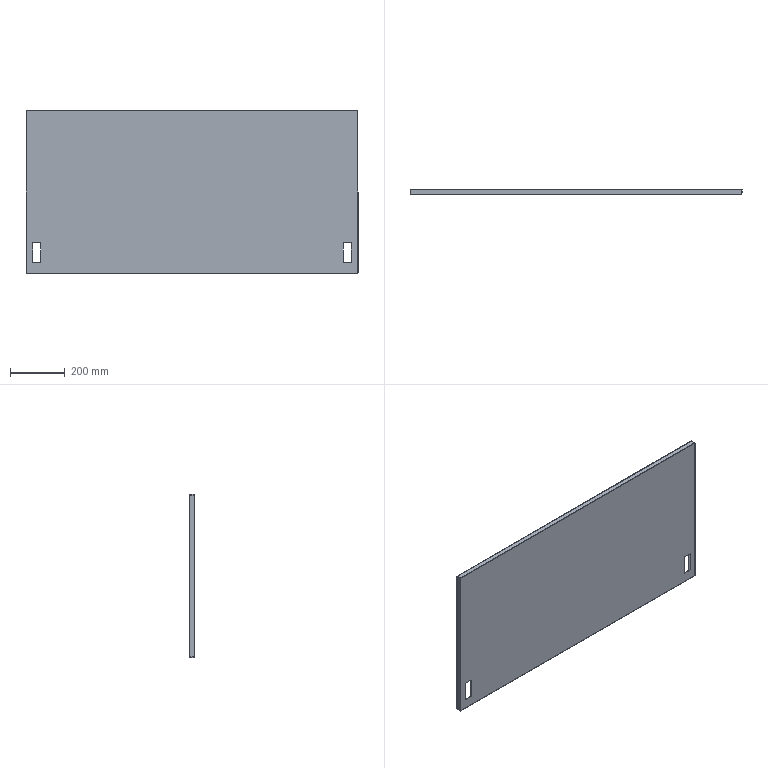Part | SolidWorks | features EdgeFlange 2, FlatPattern 1, SMBaseFlange 1, SheetMetal 1 | 1 solid | 78 faces | box 1218 x 20 x 598 mm | volume 1005424 mm3 | plane 46 | spline 16 | cylinder 16 | commonest cylinder face diameters 0.9 x8 3.3 x8